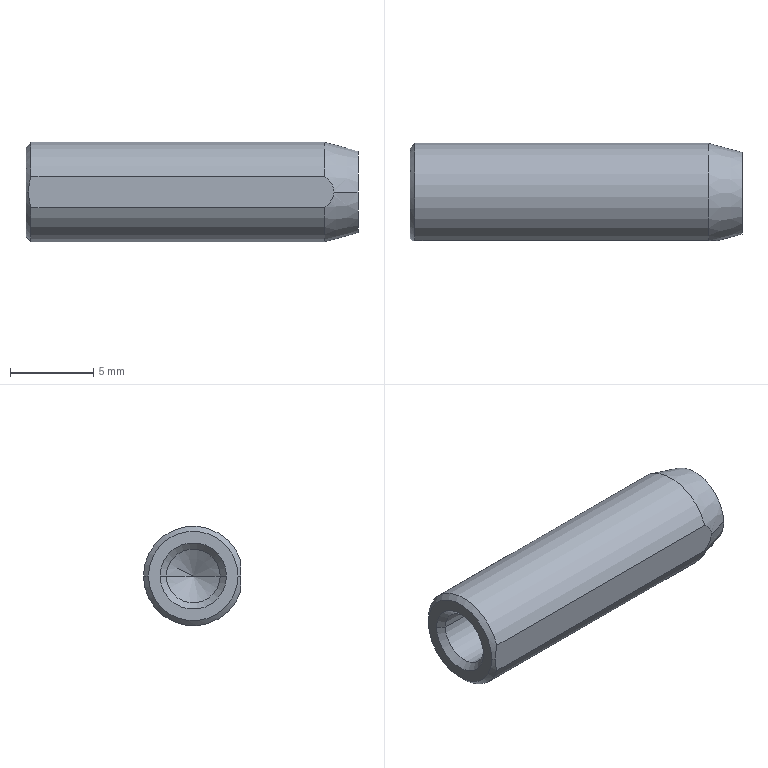Part | STEP file | MSTSS6-20-4 | 1 solid | 15 faces | box 20 x 5.85 x 6 mm | volume 470.29 mm3 | cone 8 | cylinder 4 | plane 3 | commonest cylinder face diameters 3.242 x2 6 x2
STEP:
#1=CARTESIAN_POINT('',(0.,0.,0.));
#2=DIRECTION('',(0.,0.,1.));
#3=DIRECTION('',(1.,0.,0.));
#4=AXIS2_PLACEMENT_3D('',#1,#2,#3);
#5=CARTESIAN_POINT('',(9.464,-1.621,0.));
#6=VERTEX_POINT('',#5);
#7=CARTESIAN_POINT('',(9.464,1.621,0.));
#8=VERTEX_POINT('',#7);
#9=CARTESIAN_POINT('',(9.464,0.,0.));
#10=DIRECTION('',(1.,0.,0.));
#11=DIRECTION('',(0.,1.,0.));
#12=AXIS2_PLACEMENT_3D('',#9,#10,#11);
#13=CIRCLE('',#12,1.621);
#14=CARTESIAN_POINT('',(9.464,0.,0.));
#15=DIRECTION('',(-1.,0.,0.));
#16=DIRECTION('',(0.,-1.,0.));
#17=AXIS2_PLACEMENT_3D('',#14,#15,#16);
#18=CONICAL_SURFACE('',#17,1.621,1.047);
#19=CARTESIAN_POINT('',(9.425,0.));
#20=DIRECTION('',(-1.,0.));
#21=VECTOR('',#20,1.);
#22=LINE('',#19,#21);
#23=(GEOMETRIC_REPRESENTATION_CONTEXT(2)PARAMETRIC_REPRESENTATION_CONTEXT()REPRESENTATION_CONTEXT('',''));
#24=DEFINITIONAL_REPRESENTATION('',(#22),#23);
#25=PCURVE('',#18,#24);
#26=CARTESIAN_POINT('',(10.4,0.,0.));
#27=DIRECTION('',(1.,0.,0.));
#28=DIRECTION('',(0.,1.,0.));
#29=AXIS2_PLACEMENT_3D('',#26,#27,#28);
#30=CYLINDRICAL_SURFACE('',#29,1.621);
#31=CARTESIAN_POINT('',(0.,-0.9359));
#32=DIRECTION('',(1.,0.));
#33=VECTOR('',#32,1.);
#34=LINE('',#31,#33);
#35=(GEOMETRIC_REPRESENTATION_CONTEXT(2)PARAMETRIC_REPRESENTATION_CONTEXT()REPRESENTATION_CONTEXT('',''));
#36=DEFINITIONAL_REPRESENTATION('',(#34),#35);
#37=PCURVE('',#30,#36);
#38=SURFACE_CURVE('',#13,(#25,#37),.PCURVE_S1.);
#39=EDGE_CURVE('',#6,#8,#38,.T.);
#40=ORIENTED_EDGE('',*,*,#39,.T.);
#41=CARTESIAN_POINT('',(10.4,0.,0.));
#42=VERTEX_POINT('',#41);
#43=CARTESIAN_POINT('',(9.464,1.621,0.));
#44=DIRECTION('',(-0.5,0.866,0.));
#45=VECTOR('',#44,1.);
#46=LINE('',#43,#45);
#47=CARTESIAN_POINT('',(3.142,0.));
#48=DIRECTION('',(0.,1.));
#49=VECTOR('',#48,1.);
#50=LINE('',#47,#49);
#51=(GEOMETRIC_REPRESENTATION_CONTEXT(2)PARAMETRIC_REPRESENTATION_CONTEXT()REPRESENTATION_CONTEXT('',''));
#52=DEFINITIONAL_REPRESENTATION('',(#50),#51);
#53=PCURVE('',#18,#52);
#54=CARTESIAN_POINT('',(9.464,0.,0.));
#55=DIRECTION('',(-1.,0.,0.));
#56=DIRECTION('',(0.,-1.,0.));
#57=AXIS2_PLACEMENT_3D('',#54,#55,#56);
#58=CONICAL_SURFACE('',#57,1.621,1.047);
#59=CARTESIAN_POINT('',(3.142,0.));
#60=DIRECTION('',(0.,1.));
#61=VECTOR('',#60,1.);
#62=LINE('',#59,#61);
#63=(GEOMETRIC_REPRESENTATION_CONTEXT(2)PARAMETRIC_REPRESENTATION_CONTEXT()REPRESENTATION_CONTEXT('',''));
#64=DEFINITIONAL_REPRESENTATION('',(#62),#63);
#65=PCURVE('',#58,#64);
#66=SURFACE_CURVE('',#46,(#53,#65),.PCURVE_S1.);
#67=EDGE_CURVE('',#42,#8,#66,.T.);
#68=ORIENTED_EDGE('',*,*,#67,.F.);
#69=CARTESIAN_POINT('',(9.464,-1.621,0.));
#70=DIRECTION('',(-0.5,-0.866,0.));
#71=VECTOR('',#70,1.);
#72=LINE('',#69,#71);
#73=CARTESIAN_POINT('',(6.283,0.));
#74=DIRECTION('',(0.,1.));
#75=VECTOR('',#74,1.);
#76=LINE('',#73,#75);
#77=(GEOMETRIC_REPRESENTATION_CONTEXT(2)PARAMETRIC_REPRESENTATION_CONTEXT()REPRESENTATION_CONTEXT('',''));
#78=DEFINITIONAL_REPRESENTATION('',(#76),#77);
#79=PCURVE('',#18,#78);
#80=CARTESIAN_POINT('',(0.,0.));
#81=DIRECTION('',(0.,1.));
#82=VECTOR('',#81,1.);
#83=LINE('',#80,#82);
#84=(GEOMETRIC_REPRESENTATION_CONTEXT(2)PARAMETRIC_REPRESENTATION_CONTEXT()REPRESENTATION_CONTEXT('',''));
#85=DEFINITIONAL_REPRESENTATION('',(#83),#84);
#86=PCURVE('',#58,#85);
#87=SURFACE_CURVE('',#72,(#79,#86),.PCURVE_S1.);
#88=EDGE_CURVE('',#42,#6,#87,.T.);
#89=ORIENTED_EDGE('',*,*,#88,.T.);
#90=EDGE_LOOP('',(#40,#68,#89));
#91=FACE_BOUND('',#90,.F.);
#92=ADVANCED_FACE('',(#91),#18,.F.);
#93=CARTESIAN_POINT('',(0.379,1.621,0.));
#94=VERTEX_POINT('',#93);
#95=CARTESIAN_POINT('',(10.4,1.621,0.));
#96=DIRECTION('',(1.,0.,0.));
#97=VECTOR('',#96,1.);
#98=LINE('',#95,#97);
#99=CARTESIAN_POINT('',(6.283,0.));
#100=DIRECTION('',(0.,1.));
#101=VECTOR('',#100,1.);
#102=LINE('',#99,#101);
#103=(GEOMETRIC_REPRESENTATION_CONTEXT(2)PARAMETRIC_REPRESENTATION_CONTEXT()REPRESENTATION_CONTEXT('',''));
#104=DEFINITIONAL_REPRESENTATION('',(#102),#103);
#105=PCURVE('',#30,#104);
#106=CARTESIAN_POINT('',(10.4,0.,0.));
#107=DIRECTION('',(1.,0.,0.));
#108=DIRECTION('',(0.,1.,0.));
#109=AXIS2_PLACEMENT_3D('',#106,#107,#108);
#110=CYLINDRICAL_SURFACE('',#109,1.621);
#111=CARTESIAN_POINT('',(0.,0.));
#112=DIRECTION('',(0.,1.));
#113=VECTOR('',#112,1.);
#114=LINE('',#111,#113);
#115=(GEOMETRIC_REPRESENTATION_CONTEXT(2)PARAMETRIC_REPRESENTATION_CONTEXT()REPRESENTATION_CONTEXT('',''));
#116=DEFINITIONAL_REPRESENTATION('',(#114),#115);
#117=PCURVE('',#110,#116);
#118=SURFACE_CURVE('',#98,(#105,#117),.PCURVE_S1.);
#119=EDGE_CURVE('',#94,#8,#118,.T.);
#120=ORIENTED_EDGE('',*,*,#119,.T.);
#121=ORIENTED_EDGE('',*,*,#39,.F.);
#122=CARTESIAN_POINT('',(0.379,-1.621,0.));
#123=VERTEX_POINT('',#122);
#124=CARTESIAN_POINT('',(10.4,-1.621,0.));
#125=DIRECTION('',(1.,0.,0.));
#126=VECTOR('',#125,1.);
#127=LINE('',#124,#126);
#128=CARTESIAN_POINT('',(3.142,0.));
#129=DIRECTION('',(0.,1.));
#130=VECTOR('',#129,1.);
#131=LINE('',#128,#130);
#132=(GEOMETRIC_REPRESENTATION_CONTEXT(2)PARAMETRIC_REPRESENTATION_CONTEXT()REPRESENTATION_CONTEXT('',''));
#133=DEFINITIONAL_REPRESENTATION('',(#131),#132);
#134=PCURVE('',#30,#133);
#135=CARTESIAN_POINT('',(3.142,0.));
#136=DIRECTION('',(0.,1.));
#137=VECTOR('',#136,1.);
#138=LINE('',#135,#137);
#139=(GEOMETRIC_REPRESENTATION_CONTEXT(2)PARAMETRIC_REPRESENTATION_CONTEXT()REPRESENTATION_CONTEXT('',''));
#140=DEFINITIONAL_REPRESENTATION('',(#138),#139);
#141=PCURVE('',#110,#140);
#142=SURFACE_CURVE('',#127,(#134,#141),.PCURVE_S1.);
#143=EDGE_CURVE('',#123,#6,#142,.T.);
#144=ORIENTED_EDGE('',*,*,#143,.F.);
#145=CARTESIAN_POINT('',(0.379,0.,0.));
#146=DIRECTION('',(1.,0.,0.));
#147=DIRECTION('',(0.,1.,0.));
#148=AXIS2_PLACEMENT_3D('',#145,#146,#147);
#149=CIRCLE('',#148,1.621);
#150=CARTESIAN_POINT('',(0.,-10.021));
#151=DIRECTION('',(1.,0.));
#152=VECTOR('',#151,1.);
#153=LINE('',#150,#152);
#154=(GEOMETRIC_REPRESENTATION_CONTEXT(2)PARAMETRIC_REPRESENTATION_CONTEXT()REPRESENTATION_CONTEXT('',''));
#155=DEFINITIONAL_REPRESENTATION('',(#153),#154);
#156=PCURVE('',#30,#155);
#157=CARTESIAN_POINT('',(0.,0.,0.));
#158=DIRECTION('',(-1.,0.,0.));
#159=DIRECTION('',(0.,-1.,0.));
#160=AXIS2_PLACEMENT_3D('',#157,#158,#159);
#161=CONICAL_SURFACE('',#160,2.,0.7854);
#162=CARTESIAN_POINT('',(9.425,-0.379));
#163=DIRECTION('',(-1.,0.));
#164=VECTOR('',#163,1.);
#165=LINE('',#162,#164);
#166=(GEOMETRIC_REPRESENTATION_CONTEXT(2)PARAMETRIC_REPRESENTATION_CONTEXT()REPRESENTATION_CONTEXT('',''));
#167=DEFINITIONAL_REPRESENTATION('',(#165),#166);
#168=PCURVE('',#161,#167);
#169=SURFACE_CURVE('',#149,(#156,#168),.PCURVE_S1.);
#170=EDGE_CURVE('',#123,#94,#169,.T.);
#171=ORIENTED_EDGE('',*,*,#170,.T.);
#172=EDGE_LOOP('',(#120,#121,#144,#171));
#173=FACE_BOUND('',#172,.F.);
#174=ADVANCED_FACE('',(#173),#30,.F.);
#175=CARTESIAN_POINT('',(0.,-2.,0.));
#176=VERTEX_POINT('',#175);
#177=CARTESIAN_POINT('',(0.,-2.,0.));
#178=DIRECTION('',(-0.7071,-0.7071,0.));
#179=VECTOR('',#178,1.);
#180=LINE('',#177,#179);
#181=CARTESIAN_POINT('',(6.283,0.));
#182=DIRECTION('',(0.,1.));
#183=VECTOR('',#182,1.);
#184=LINE('',#181,#183);
#185=(GEOMETRIC_REPRESENTATION_CONTEXT(2)PARAMETRIC_REPRESENTATION_CONTEXT()REPRESENTATION_CONTEXT('',''));
#186=DEFINITIONAL_REPRESENTATION('',(#184),#185);
#187=PCURVE('',#161,#186);
#188=CARTESIAN_POINT('',(0.,0.,0.));
#189=DIRECTION('',(-1.,0.,0.));
#190=DIRECTION('',(0.,-1.,0.));
#191=AXIS2_PLACEMENT_3D('',#188,#189,#190);
#192=CONICAL_SURFACE('',#191,2.,0.7854);
#193=CARTESIAN_POINT('',(0.,0.));
#194=DIRECTION('',(0.,1.));
#195=VECTOR('',#194,1.);
#196=LINE('',#193,#195);
#197=(GEOMETRIC_REPRESENTATION_CONTEXT(2)PARAMETRIC_REPRESENTATION_CONTEXT()REPRESENTATION_CONTEXT('',''));
#198=DEFINITIONAL_REPRESENTATION('',(#196),#197);
#199=PCURVE('',#192,#198);
#200=SURFACE_CURVE('',#180,(#187,#199),.PCURVE_S1.);
#201=EDGE_CURVE('',#123,#176,#200,.T.);
#202=ORIENTED_EDGE('',*,*,#201,.T.);
#203=CARTESIAN_POINT('',(0.,2.,0.));
#204=VERTEX_POINT('',#203);
#205=CARTESIAN_POINT('',(0.,0.,0.));
#206=DIRECTION('',(1.,0.,0.));
#207=DIRECTION('',(0.,1.,0.));
#208=AXIS2_PLACEMENT_3D('',#205,#206,#207);
#209=CIRCLE('',#208,2.);
#210=CARTESIAN_POINT('',(9.425,0.));
#211=DIRECTION('',(-1.,0.));
#212=VECTOR('',#211,1.);
#213=LINE('',#210,#212);
#214=(GEOMETRIC_REPRESENTATION_CONTEXT(2)PARAMETRIC_REPRESENTATION_CONTEXT()REPRESENTATION_CONTEXT('',''));
#215=DEFINITIONAL_REPRESENTATION('',(#213),#214);
#216=PCURVE('',#161,#215);
#217=CARTESIAN_POINT('',(0.,0.,0.));
#218=DIRECTION('',(1.,0.,0.));
#219=DIRECTION('',(0.,1.,0.));
#220=AXIS2_PLACEMENT_3D('',#217,#218,#219);
#221=PLANE('',#220);
#222=CARTESIAN_POINT('',(0.,0.));
#223=DIRECTION('',(1.,0.));
#224=AXIS2_PLACEMENT_2D('',#222,#223);
#225=CIRCLE('',#224,2.);
#226=(GEOMETRIC_REPRESENTATION_CONTEXT(2)PARAMETRIC_REPRESENTATION_CONTEXT()REPRESENTATION_CONTEXT('',''));
#227=DEFINITIONAL_REPRESENTATION('',(#225),#226);
#228=PCURVE('',#221,#227);
#229=SURFACE_CURVE('',#209,(#216,#228),.PCURVE_S1.);
#230=EDGE_CURVE('',#176,#204,#229,.T.);
#231=ORIENTED_EDGE('',*,*,#230,.T.);
#232=CARTESIAN_POINT('',(0.,2.,0.));
#233=DIRECTION('',(-0.7071,0.7071,0.));
#234=VECTOR('',#233,1.);
#235=LINE('',#232,#234);
#236=CARTESIAN_POINT('',(3.142,0.));
#237=DIRECTION('',(0.,1.));
#238=VECTOR('',#237,1.);
#239=LINE('',#236,#238);
#240=(GEOMETRIC_REPRESENTATION_CONTEXT(2)PARAMETRIC_REPRESENTATION_CONTEXT()REPRESENTATION_CONTEXT('',''));
#241=DEFINITIONAL_REPRESENTATION('',(#239),#240);
#242=PCURVE('',#161,#241);
#243=CARTESIAN_POINT('',(3.142,0.));
#244=DIRECTION('',(0.,1.));
#245=VECTOR('',#244,1.);
#246=LINE('',#243,#245);
#247=(GEOMETRIC_REPRESENTATION_CONTEXT(2)PARAMETRIC_REPRESENTATION_CONTEXT()REPRESENTATION_CONTEXT('',''));
#248=DEFINITIONAL_REPRESENTATION('',(#246),#247);
#249=PCURVE('',#192,#248);
#250=SURFACE_CURVE('',#235,(#242,#249),.PCURVE_S1.);
#251=EDGE_CURVE('',#94,#204,#250,.T.);
#252=ORIENTED_EDGE('',*,*,#251,.F.);
#253=ORIENTED_EDGE('',*,*,#170,.F.);
#254=EDGE_LOOP('',(#202,#231,#252,#253));
#255=FACE_BOUND('',#254,.F.);
#256=ADVANCED_FACE('',(#255),#161,.F.);
#257=CARTESIAN_POINT('',(20.,2.464,0.));
#258=VERTEX_POINT('',#257);
#259=CARTESIAN_POINT('',(20.,-2.464,0.));
#260=VERTEX_POINT('',#259);
#261=CARTESIAN_POINT('',(20.,0.,0.));
#262=DIRECTION('',(1.,0.,0.));
#263=DIRECTION('',(0.,1.,0.));
#264=AXIS2_PLACEMENT_3D('',#261,#262,#263);
#265=CIRCLE('',#264,2.464);
#266=CARTESIAN_POINT('',(18.,0.,0.));
#267=DIRECTION('',(-1.,0.,0.));
#268=DIRECTION('',(0.,-1.,0.));
#269=AXIS2_PLACEMENT_3D('',#266,#267,#268);
#270=CONICAL_SURFACE('',#269,3.,0.2618);
#271=CARTESIAN_POINT('',(3.142,-2.));
#272=DIRECTION('',(-1.,0.));
#273=VECTOR('',#272,1.);
#274=LINE('',#271,#273);
#275=(GEOMETRIC_REPRESENTATION_CONTEXT(2)PARAMETRIC_REPRESENTATION_CONTEXT()REPRESENTATION_CONTEXT('',''));
#276=DEFINITIONAL_REPRESENTATION('',(#274),#275);
#277=PCURVE('',#270,#276);
#278=CARTESIAN_POINT('',(20.,0.,2.464));
#279=DIRECTION('',(-1.,0.,0.));
#280=DIRECTION('',(0.,-1.,0.));
#281=AXIS2_PLACEMENT_3D('',#278,#279,#280);
#282=PLANE('',#281);
#283=CARTESIAN_POINT('',(-2.464,-2.464));
#284=CARTESIAN_POINT('',(-2.464,1.804));
#285=CARTESIAN_POINT('',(1.232,-0.3301));
#286=CARTESIAN_POINT('',(4.928,-2.464));
#287=CARTESIAN_POINT('',(1.232,-4.598));
#288=CARTESIAN_POINT('',(-2.464,-6.732));
#289=CARTESIAN_POINT('',(-2.464,-2.464));
#290=(BOUNDED_CURVE()B_SPLINE_CURVE(2,(#283,#284,#285,#286,#287,#288,#289),.UNSPECIFIED.,.T.,.F.)B_SPLINE_CURVE_WITH_KNOTS((1,2,2,2,2,1),(-2.094,0.,2.094,4.189,6.283,8.378),.UNSPECIFIED.)CURVE()GEOMETRIC_REPRESENTATION_ITEM()RATIONAL_B_SPLINE_CURVE((1.,0.5,1.,0.5,1.,0.5,1.))REPRESENTATION_ITEM(''));
#291=(GEOMETRIC_REPRESENTATION_CONTEXT(2)PARAMETRIC_REPRESENTATION_CONTEXT()REPRESENTATION_CONTEXT('',''));
#292=DEFINITIONAL_REPRESENTATION('',(#290),#291);
#293=PCURVE('',#282,#292);
#294=SURFACE_CURVE('',#265,(#277,#293),.PCURVE_S1.);
#295=EDGE_CURVE('',#258,#260,#294,.T.);
#296=ORIENTED_EDGE('',*,*,#295,.F.);
#297=CARTESIAN_POINT('',(18.,3.,0.));
#298=VERTEX_POINT('',#297);
#299=CARTESIAN_POINT('',(18.,3.,0.));
#300=DIRECTION('',(-0.9659,0.2588,0.));
#301=VECTOR('',#300,1.);
#302=LINE('',#299,#301);
#303=CARTESIAN_POINT('',(3.142,0.));
#304=DIRECTION('',(0.,1.));
#305=VECTOR('',#304,1.);
#306=LINE('',#303,#305);
#307=(GEOMETRIC_REPRESENTATION_CONTEXT(2)PARAMETRIC_REPRESENTATION_CONTEXT()REPRESENTATION_CONTEXT('',''));
#308=DEFINITIONAL_REPRESENTATION('',(#306),#307);
#309=PCURVE('',#270,#308);
#310=CARTESIAN_POINT('',(18.,0.,0.));
#311=DIRECTION('',(-1.,0.,0.));
#312=DIRECTION('',(0.,-1.,0.));
#313=AXIS2_PLACEMENT_3D('',#310,#311,#312);
#314=CONICAL_SURFACE('',#313,3.,0.2618);
#315=CARTESIAN_POINT('',(3.142,0.));
#316=DIRECTION('',(0.,1.));
#317=VECTOR('',#316,1.);
#318=LINE('',#315,#317);
#319=(GEOMETRIC_REPRESENTATION_CONTEXT(2)PARAMETRIC_REPRESENTATION_CONTEXT()REPRESENTATION_CONTEXT('',''));
#320=DEFINITIONAL_REPRESENTATION('',(#318),#319);
#321=PCURVE('',#314,#320);
#322=SURFACE_CURVE('',#302,(#309,#321),.PCURVE_S1.);
#323=EDGE_CURVE('',#258,#298,#322,.T.);
#324=ORIENTED_EDGE('',*,*,#323,.T.);
#325=CARTESIAN_POINT('',(18.,-2.85,0.9367));
#326=VERTEX_POINT('',#325);
#327=CARTESIAN_POINT('',(18.,0.,0.));
#328=DIRECTION('',(1.,0.,0.));
#329=DIRECTION('',(0.,1.,0.));
#330=AXIS2_PLACEMENT_3D('',#327,#328,#329);
#331=CIRCLE('',#330,3.);
#332=CARTESIAN_POINT('',(3.142,0.));
#333=DIRECTION('',(-1.,0.));
#334=VECTOR('',#333,1.);
#335=LINE('',#332,#334);
#336=(GEOMETRIC_REPRESENTATION_CONTEXT(2)PARAMETRIC_REPRESENTATION_CONTEXT()REPRESENTATION_CONTEXT('',''));
#337=DEFINITIONAL_REPRESENTATION('',(#335),#336);
#338=PCURVE('',#270,#337);
#339=CARTESIAN_POINT('',(20.,0.,0.));
#340=DIRECTION('',(1.,0.,0.));
#341=DIRECTION('',(0.,1.,0.));
#342=AXIS2_PLACEMENT_3D('',#339,#340,#341);
#343=CYLINDRICAL_SURFACE('',#342,3.);
#344=CARTESIAN_POINT('',(0.,-2.));
#345=DIRECTION('',(1.,0.));
#346=VECTOR('',#345,1.);
#347=LINE('',#344,#346);
#348=(GEOMETRIC_REPRESENTATION_CONTEXT(2)PARAMETRIC_REPRESENTATION_CONTEXT()REPRESENTATION_CONTEXT('',''));
#349=DEFINITIONAL_REPRESENTATION('',(#347),#348);
#350=PCURVE('',#343,#349);
#351=SURFACE_CURVE('',#331,(#338,#350),.PCURVE_S1.);
#352=EDGE_CURVE('',#298,#326,#351,.T.);
#353=ORIENTED_EDGE('',*,*,#352,.T.);
#354=CARTESIAN_POINT('',(18.56,-2.85,0.));
#355=VERTEX_POINT('',#354);
#356=CARTESIAN_POINT('',(18.56,-2.85,0.));
#357=CARTESIAN_POINT('',(18.56,-2.85,0.0942));
#358=CARTESIAN_POINT('',(18.542,-2.85,0.1877));
#359=CARTESIAN_POINT('',(18.478,-2.85,0.365));
#360=CARTESIAN_POINT('',(18.433,-2.85,0.4473));
#361=CARTESIAN_POINT('',(18.275,-2.85,0.682));
#362=CARTESIAN_POINT('',(18.142,-2.85,0.8146));
#363=CARTESIAN_POINT('',(18.,-2.85,0.9367));
#364=B_SPLINE_CURVE_WITH_KNOTS('',3,(#356,#357,#358,#359,#360,#361,#362,#363),.UNSPECIFIED.,.F.,.F.,(4,2,2,4),(0.008062,0.008341,0.00862,0.009177),.UNSPECIFIED.);
#365=CARTESIAN_POINT('',(0.,-0.5598));
#366=CARTESIAN_POINT('',(0.00601,-0.5598));
#367=CARTESIAN_POINT('',(0.01801,-0.5586));
#368=CARTESIAN_POINT('',(0.03591,-0.5534));
#369=CARTESIAN_POINT('',(0.05362,-0.545));
#370=CARTESIAN_POINT('',(0.0711,-0.5333));
#371=CARTESIAN_POINT('',(0.08827,-0.5188));
#372=CARTESIAN_POINT('',(0.1051,-0.5013));
#373=CARTESIAN_POINT('',(0.1214,-0.4814));
#374=CARTESIAN_POINT('',(0.1373,-0.4593));
#375=CARTESIAN_POINT('',(0.1527,-0.435));
#376=CARTESIAN_POINT('',(0.1678,-0.4088));
#377=CARTESIAN_POINT('',(0.1824,-0.3807));
#378=CARTESIAN_POINT('',(0.1967,-0.3511));
#379=CARTESIAN_POINT('',(0.2105,-0.3204));
#380=CARTESIAN_POINT('',(0.2238,-0.2884));
#381=CARTESIAN_POINT('',(0.2368,-0.2554));
#382=CARTESIAN_POINT('',(0.2493,-0.2214));
#383=CARTESIAN_POINT('',(0.2615,-0.1864));
#384=CARTESIAN_POINT('',(0.2733,-0.1506));
#385=CARTESIAN_POINT('',(0.2848,-0.114));
#386=CARTESIAN_POINT('',(0.296,-0.07662));
#387=CARTESIAN_POINT('',(0.3069,-0.03864));
#388=CARTESIAN_POINT('',(0.314,-0.01294));
#389=CARTESIAN_POINT('',(0.3176,0.));
#390=B_SPLINE_CURVE_WITH_KNOTS('',3,(#365,#366,#367,#368,#369,#370,#371,#372,#373,#374,#375,#376,#377,#378,#379,#380,#381,#382,#383,#384,#385,#386,#387,#388,#389),.UNSPECIFIED.,.F.,.F.,(4,1,1,1,1,1,1,1,1,1,1,1,1,1,1,1,1,1,1,1,1,1,4),(0.008062,0.008113,0.008163,0.008214,0.008265,0.008316,0.008366,0.008417,0.008468,0.008518,0.008569,0.00862,0.00867,0.008721,0.008772,0.008822,0.008873,0.008924,0.008974,0.009025,0.009076,0.009126,0.009177),.QUASI_UNIFORM_KNOTS.);
#391=(GEOMETRIC_REPRESENTATION_CONTEXT(2)PARAMETRIC_REPRESENTATION_CONTEXT()REPRESENTATION_CONTEXT('',''));
#392=DEFINITIONAL_REPRESENTATION('',(#390),#391);
#393=PCURVE('',#270,#392);
#394=CARTESIAN_POINT('',(20.,-2.85,-3.));
#395=DIRECTION('',(0.,-1.,0.));
#396=DIRECTION('',(1.,0.,0.));
#397=AXIS2_PLACEMENT_3D('',#394,#395,#396);
#398=PLANE('',#397);
#399=CARTESIAN_POINT('',(-1.44,3.));
#400=CARTESIAN_POINT('',(-1.44,3.094));
#401=CARTESIAN_POINT('',(-1.458,3.188));
#402=CARTESIAN_POINT('',(-1.522,3.365));
#403=CARTESIAN_POINT('',(-1.567,3.447));
#404=CARTESIAN_POINT('',(-1.725,3.682));
#405=CARTESIAN_POINT('',(-1.858,3.815));
#406=CARTESIAN_POINT('',(-2.,3.937));
#407=B_SPLINE_CURVE_WITH_KNOTS('',3,(#399,#400,#401,#402,#403,#404,#405,#406),.UNSPECIFIED.,.F.,.F.,(4,2,2,4),(0.008062,0.008341,0.00862,0.009177),.UNSPECIFIED.);
#408=(GEOMETRIC_REPRESENTATION_CONTEXT(2)PARAMETRIC_REPRESENTATION_CONTEXT()REPRESENTATION_CONTEXT('',''));
#409=DEFINITIONAL_REPRESENTATION('',(#407),#408);
#410=PCURVE('',#398,#409);
#411=SURFACE_CURVE('',#364,(#393,#410),.PCURVE_S1.);
#412=EDGE_CURVE('',#355,#326,#411,.T.);
#413=ORIENTED_EDGE('',*,*,#412,.F.);
#414=CARTESIAN_POINT('',(18.,-3.,0.));
#415=DIRECTION('',(-0.9659,-0.2588,0.));
#416=VECTOR('',#415,1.);
#417=LINE('',#414,#416);
#418=CARTESIAN_POINT('',(0.,0.));
#419=DIRECTION('',(0.,1.));
#420=VECTOR('',#419,1.);
#421=LINE('',#418,#420);
#422=(GEOMETRIC_REPRESENTATION_CONTEXT(2)PARAMETRIC_REPRESENTATION_CONTEXT()REPRESENTATION_CONTEXT('',''));
#423=DEFINITIONAL_REPRESENTATION('',(#421),#422);
#424=PCURVE('',#270,#423);
#425=CARTESIAN_POINT('',(6.283,0.));
#426=DIRECTION('',(0.,1.));
#427=VECTOR('',#426,1.);
#428=LINE('',#425,#427);
#429=(GEOMETRIC_REPRESENTATION_CONTEXT(2)PARAMETRIC_REPRESENTATION_CONTEXT()REPRESENTATION_CONTEXT('',''));
#430=DEFINITIONAL_REPRESENTATION('',(#428),#429);
#431=PCURVE('',#314,#430);
#432=SURFACE_CURVE('',#417,(#424,#431),.PCURVE_S1.);
#433=EDGE_CURVE('',#260,#355,#432,.T.);
#434=ORIENTED_EDGE('',*,*,#433,.F.);
#435=EDGE_LOOP('',(#296,#324,#353,#413,#434));
#436=FACE_BOUND('',#435,.T.);
#437=ADVANCED_FACE('',(#436),#270,.T.);
#438=CARTESIAN_POINT('',(0.3,-2.85,-0.9367));
#439=VERTEX_POINT('',#438);
#440=CARTESIAN_POINT('',(0.3,3.,0.));
#441=VERTEX_POINT('',#440);
#442=CARTESIAN_POINT('',(0.3,0.,0.));
#443=DIRECTION('',(1.,0.,0.));
#444=DIRECTION('',(0.,1.,0.));
#445=AXIS2_PLACEMENT_3D('',#442,#443,#444);
#446=CIRCLE('',#445,3.);
#447=CARTESIAN_POINT('',(20.,0.,0.));
#448=DIRECTION('',(1.,0.,0.));
#449=DIRECTION('',(0.,1.,0.));
#450=AXIS2_PLACEMENT_3D('',#447,#448,#449);
#451=CYLINDRICAL_SURFACE('',#450,3.);
#452=CARTESIAN_POINT('',(0.,-19.7));
#453=DIRECTION('',(1.,0.));
#454=VECTOR('',#453,1.);
#455=LINE('',#452,#454);
#456=(GEOMETRIC_REPRESENTATION_CONTEXT(2)PARAMETRIC_REPRESENTATION_CONTEXT()REPRESENTATION_CONTEXT('',''));
#457=DEFINITIONAL_REPRESENTATION('',(#455),#456);
#458=PCURVE('',#451,#457);
#459=CARTESIAN_POINT('',(0.,0.,0.));
#460=DIRECTION('',(1.,0.,0.));
#461=DIRECTION('',(0.,1.,0.));
#462=AXIS2_PLACEMENT_3D('',#459,#460,#461);
#463=CONICAL_SURFACE('',#462,2.7,0.7854);
#464=CARTESIAN_POINT('',(0.,0.3));
#465=DIRECTION('',(1.,0.));
#466=VECTOR('',#465,1.);
#467=LINE('',#464,#466);
#468=(GEOMETRIC_REPRESENTATION_CONTEXT(2)PARAMETRIC_REPRESENTATION_CONTEXT()REPRESENTATION_CONTEXT('',''));
#469=DEFINITIONAL_REPRESENTATION('',(#467),#468);
#470=PCURVE('',#463,#469);
#471=SURFACE_CURVE('',#446,(#458,#470),.PCURVE_S1.);
#472=EDGE_CURVE('',#439,#441,#471,.T.);
#473=ORIENTED_EDGE('',*,*,#472,.T.);
#474=CARTESIAN_POINT('',(20.,3.,0.));
#475=DIRECTION('',(1.,0.,0.));
#476=VECTOR('',#475,1.);
#477=LINE('',#474,#476);
#478=CARTESIAN_POINT('',(6.283,0.));
#479=DIRECTION('',(0.,1.));
#480=VECTOR('',#479,1.);
#481=LINE('',#478,#480);
#482=(GEOMETRIC_REPRESENTATION_CONTEXT(2)PARAMETRIC_REPRESENTATION_CONTEXT()REPRESENTATION_CONTEXT('',''));
#483=DEFINITIONAL_REPRESENTATION('',(#481),#482);
#484=PCURVE('',#451,#483);
#485=CARTESIAN_POINT('',(0.,0.));
#486=DIRECTION('',(0.,1.));
#487=VECTOR('',#486,1.);
#488=LINE('',#485,#487);
#489=(GEOMETRIC_REPRESENTATION_CONTEXT(2)PARAMETRIC_REPRESENTATION_CONTEXT()REPRESENTATION_CONTEXT('',''));
#490=DEFINITIONAL_REPRESENTATION('',(#488),#489);
#491=PCURVE('',#343,#490);
#492=SURFACE_CURVE('',#477,(#484,#491),.PCURVE_S1.);
#493=EDGE_CURVE('',#441,#298,#492,.T.);
#494=ORIENTED_EDGE('',*,*,#493,.T.);
#495=CARTESIAN_POINT('',(18.,-2.85,-0.9367));
#496=VERTEX_POINT('',#495);
#497=CARTESIAN_POINT('',(18.,0.,0.));
#498=DIRECTION('',(1.,0.,0.));
#499=DIRECTION('',(0.,1.,0.));
#500=AXIS2_PLACEMENT_3D('',#497,#498,#499);
#501=CIRCLE('',#500,3.);
#502=CARTESIAN_POINT('',(0.,-2.));
#503=DIRECTION('',(1.,0.));
#504=VECTOR('',#503,1.);
#505=LINE('',#502,#504);
#506=(GEOMETRIC_REPRESENTATION_CONTEXT(2)PARAMETRIC_REPRESENTATION_CONTEXT()REPRESENTATION_CONTEXT('',''));
#507=DEFINITIONAL_REPRESENTATION('',(#505),#506);
#508=PCURVE('',#451,#507);
#509=CARTESIAN_POINT('',(9.425,0.));
#510=DIRECTION('',(-1.,0.));
#511=VECTOR('',#510,1.);
#512=LINE('',#509,#511);
#513=(GEOMETRIC_REPRESENTATION_CONTEXT(2)PARAMETRIC_REPRESENTATION_CONTEXT()REPRESENTATION_CONTEXT('',''));
#514=DEFINITIONAL_REPRESENTATION('',(#512),#513);
#515=PCURVE('',#314,#514);
#516=SURFACE_CURVE('',#501,(#508,#515),.PCURVE_S1.);
#517=EDGE_CURVE('',#496,#298,#516,.T.);
#518=ORIENTED_EDGE('',*,*,#517,.F.);
#519=CARTESIAN_POINT('',(20.,-2.85,-0.9367));
#520=DIRECTION('',(1.,0.,0.));
#521=VECTOR('',#520,1.);
#522=LINE('',#519,#521);
#523=CARTESIAN_POINT('',(3.459,0.));
#524=DIRECTION('',(0.,1.));
#525=VECTOR('',#524,1.);
#526=LINE('',#523,#525);
#527=(GEOMETRIC_REPRESENTATION_CONTEXT(2)PARAMETRIC_REPRESENTATION_CONTEXT()REPRESENTATION_CONTEXT('',''));
#528=DEFINITIONAL_REPRESENTATION('',(#526),#527);
#529=PCURVE('',#451,#528);
#530=CARTESIAN_POINT('',(0.,2.063));
#531=DIRECTION('',(1.,0.));
#532=VECTOR('',#531,1.);
#533=LINE('',#530,#532);
#534=(GEOMETRIC_REPRESENTATION_CONTEXT(2)PARAMETRIC_REPRESENTATION_CONTEXT()REPRESENTATION_CONTEXT('',''));
#535=DEFINITIONAL_REPRESENTATION('',(#533),#534);
#536=PCURVE('',#398,#535);
#537=SURFACE_CURVE('',#522,(#529,#536),.PCURVE_S1.);
#538=EDGE_CURVE('',#439,#496,#537,.T.);
#539=ORIENTED_EDGE('',*,*,#538,.F.);
#540=EDGE_LOOP('',(#473,#494,#518,#539));
#541=FACE_BOUND('',#540,.T.);
#542=ADVANCED_FACE('',(#541),#451,.T.);
#543=CARTESIAN_POINT('',(0.,2.7,0.));
#544=VERTEX_POINT('',#543);
#545=CARTESIAN_POINT('',(0.,-2.7,0.));
#546=VERTEX_POINT('',#545);
#547=CARTESIAN_POINT('',(0.,0.,0.));
#548=DIRECTION('',(1.,0.,0.));
#549=DIRECTION('',(0.,1.,0.));
#550=AXIS2_PLACEMENT_3D('',#547,#548,#549);
#551=CIRCLE('',#550,2.7);
#552=CARTESIAN_POINT('',(0.,0.,0.));
#553=DIRECTION('',(1.,0.,0.));
#554=DIRECTION('',(0.,1.,0.));
#555=AXIS2_PLACEMENT_3D('',#552,#553,#554);
#556=CONICAL_SURFACE('',#555,2.7,0.7854);
#557=CARTESIAN_POINT('',(0.,0.));
#558=DIRECTION('',(1.,0.));
#559=VECTOR('',#558,1.);
#560=LINE('',#557,#559);
#561=(GEOMETRIC_REPRESENTATION_CONTEXT(2)PARAMETRIC_REPRESENTATION_CONTEXT()REPRESENTATION_CONTEXT('',''));
#562=DEFINITIONAL_REPRESENTATION('',(#560),#561);
#563=PCURVE('',#556,#562);
#564=CARTESIAN_POINT('',(0.,0.));
#565=DIRECTION('',(1.,0.));
#566=AXIS2_PLACEMENT_2D('',#564,#565);
#567=CIRCLE('',#566,2.7);
#568=(GEOMETRIC_REPRESENTATION_CONTEXT(2)PARAMETRIC_REPRESENTATION_CONTEXT()REPRESENTATION_CONTEXT('',''));
#569=DEFINITIONAL_REPRESENTATION('',(#567),#568);
#570=PCURVE('',#221,#569);
#571=SURFACE_CURVE('',#551,(#563,#570),.PCURVE_S1.);
#572=EDGE_CURVE('',#544,#546,#571,.T.);
#573=ORIENTED_EDGE('',*,*,#572,.T.);
#574=CARTESIAN_POINT('',(0.15,-2.85,0.));
#575=VERTEX_POINT('',#574);
#576=CARTESIAN_POINT('',(0.,-2.7,0.));
#577=DIRECTION('',(0.7071,-0.7071,0.));
#578=VECTOR('',#577,1.);
#579=LINE('',#576,#578);
#580=CARTESIAN_POINT('',(3.142,0.));
#581=DIRECTION('',(0.,1.));
#582=VECTOR('',#581,1.);
#583=LINE('',#580,#582);
#584=(GEOMETRIC_REPRESENTATION_CONTEXT(2)PARAMETRIC_REPRESENTATION_CONTEXT()REPRESENTATION_CONTEXT('',''));
#585=DEFINITIONAL_REPRESENTATION('',(#583),#584);
#586=PCURVE('',#556,#585);
#587=CARTESIAN_POINT('',(3.142,0.));
#588=DIRECTION('',(0.,1.));
#589=VECTOR('',#588,1.);
#590=LINE('',#587,#589);
#591=(GEOMETRIC_REPRESENTATION_CONTEXT(2)PARAMETRIC_REPRESENTATION_CONTEXT()REPRESENTATION_CONTEXT('',''));
#592=DEFINITIONAL_REPRESENTATION('',(#590),#591);
#593=PCURVE('',#463,#592);
#594=SURFACE_CURVE('',#579,(#586,#593),.PCURVE_S1.);
#595=EDGE_CURVE('',#546,#575,#594,.T.);
#596=ORIENTED_EDGE('',*,*,#595,.T.);
#597=CARTESIAN_POINT('',(0.3,-2.85,0.9367));
#598=VERTEX_POINT('',#597);
#599=CARTESIAN_POINT('',(0.3,-2.85,0.9367));
#600=CARTESIAN_POINT('',(0.205,-2.85,0.6325));
#601=CARTESIAN_POINT('',(0.15,-2.85,0.3209));
#602=CARTESIAN_POINT('',(0.15,-2.85,0.));
#603=B_SPLINE_CURVE_WITH_KNOTS('',3,(#599,#600,#601,#602),.UNSPECIFIED.,.F.,.F.,(4,4),(0.009751,0.01068),.PIECEWISE_BEZIER_KNOTS.);
#604=CARTESIAN_POINT('',(2.824,0.3));
#605=CARTESIAN_POINT('',(2.828,0.2957));
#606=CARTESIAN_POINT('',(2.837,0.2872));
#607=CARTESIAN_POINT('',(2.851,0.275));
#608=CARTESIAN_POINT('',(2.864,0.2633));
#609=CARTESIAN_POINT('',(2.878,0.2521));
#610=CARTESIAN_POINT('',(2.891,0.2415));
#611=CARTESIAN_POINT('',(2.905,0.2314));
#612=CARTESIAN_POINT('',(2.919,0.2218));
#613=CARTESIAN_POINT('',(2.933,0.2128));
#614=CARTESIAN_POINT('',(2.948,0.2044));
#615=CARTESIAN_POINT('',(2.962,0.1965));
#616=CARTESIAN_POINT('',(2.977,0.1892));
#617=CARTESIAN_POINT('',(2.991,0.1825));
#618=CARTESIAN_POINT('',(3.006,0.1764));
#619=CARTESIAN_POINT('',(3.021,0.1709));
#620=CARTESIAN_POINT('',(3.035,0.1661));
#621=CARTESIAN_POINT('',(3.05,0.1618));
#622=CARTESIAN_POINT('',(3.065,0.1582));
#623=CARTESIAN_POINT('',(3.081,0.1552));
#624=CARTESIAN_POINT('',(3.096,0.1529));
#625=CARTESIAN_POINT('',(3.111,0.1512));
#626=CARTESIAN_POINT('',(3.126,0.1502));
#627=CARTESIAN_POINT('',(3.136,0.15));
#628=CARTESIAN_POINT('',(3.142,0.15));
#629=B_SPLINE_CURVE_WITH_KNOTS('',3,(#604,#605,#606,#607,#608,#609,#610,#611,#612,#613,#614,#615,#616,#617,#618,#619,#620,#621,#622,#623,#624,#625,#626,#627,#628),.UNSPECIFIED.,.F.,.F.,(4,1,1,1,1,1,1,1,1,1,1,1,1,1,1,1,1,1,1,1,1,1,4),(0.009751,0.009793,0.009835,0.009877,0.00992,0.009962,0.01,0.01005,0.01009,0.01013,0.01017,0.01022,0.01026,0.0103,0.01034,0.01038,0.01043,0.01047,0.01051,0.01055,0.0106,0.01064,0.01068),.QUASI_UNIFORM_KNOTS.);
#630=(GEOMETRIC_REPRESENTATION_CONTEXT(2)PARAMETRIC_REPRESENTATION_CONTEXT()REPRESENTATION_CONTEXT('',''));
#631=DEFINITIONAL_REPRESENTATION('',(#629),#630);
#632=PCURVE('',#556,#631);
#633=CARTESIAN_POINT('',(-19.7,3.937));
#634=CARTESIAN_POINT('',(-19.795,3.632));
#635=CARTESIAN_POINT('',(-19.85,3.321));
#636=CARTESIAN_POINT('',(-19.85,3.));
#637=B_SPLINE_CURVE_WITH_KNOTS('',3,(#633,#634,#635,#636),.UNSPECIFIED.,.F.,.F.,(4,4),(0.009751,0.01068),.PIECEWISE_BEZIER_KNOTS.);
#638=(GEOMETRIC_REPRESENTATION_CONTEXT(2)PARAMETRIC_REPRESENTATION_CONTEXT()REPRESENTATION_CONTEXT('',''));
#639=DEFINITIONAL_REPRESENTATION('',(#637),#638);
#640=PCURVE('',#398,#639);
#641=SURFACE_CURVE('',#603,(#632,#640),.PCURVE_S1.);
#642=EDGE_CURVE('',#598,#575,#641,.T.);
#643=ORIENTED_EDGE('',*,*,#642,.F.);
#644=CARTESIAN_POINT('',(0.3,0.,0.));
#645=DIRECTION('',(1.,0.,0.));
#646=DIRECTION('',(0.,1.,0.));
#647=AXIS2_PLACEMENT_3D('',#644,#645,#646);
#648=CIRCLE('',#647,3.);
#649=CARTESIAN_POINT('',(0.,0.3));
#650=DIRECTION('',(1.,0.));
#651=VECTOR('',#650,1.);
#652=LINE('',#649,#651);
#653=(GEOMETRIC_REPRESENTATION_CONTEXT(2)PARAMETRIC_REPRESENTATION_CONTEXT()REPRESENTATION_CONTEXT('',''));
#654=DEFINITIONAL_REPRESENTATION('',(#652),#653);
#655=PCURVE('',#556,#654);
#656=CARTESIAN_POINT('',(0.,-19.7));
#657=DIRECTION('',(1.,0.));
#658=VECTOR('',#657,1.);
#659=LINE('',#656,#658);
#660=(GEOMETRIC_REPRESENTATION_CONTEXT(2)PARAMETRIC_REPRESENTATION_CONTEXT()REPRESENTATION_CONTEXT('',''));
#661=DEFINITIONAL_REPRESENTATION('',(#659),#660);
#662=PCURVE('',#343,#661);
#663=SURFACE_CURVE('',#648,(#655,#662),.PCURVE_S1.);
#664=EDGE_CURVE('',#441,#598,#663,.T.);
#665=ORIENTED_EDGE('',*,*,#664,.F.);
#666=CARTESIAN_POINT('',(0.,2.7,0.));
#667=DIRECTION('',(0.7071,0.7071,0.));
#668=VECTOR('',#667,1.);
#669=LINE('',#666,#668);
#670=CARTESIAN_POINT('',(0.,0.));
#671=DIRECTION('',(0.,1.));
#672=VECTOR('',#671,1.);
#673=LINE('',#670,#672);
#674=(GEOMETRIC_REPRESENTATION_CONTEXT(2)PARAMETRIC_REPRESENTATION_CONTEXT()REPRESENTATION_CONTEXT('',''));
#675=DEFINITIONAL_REPRESENTATION('',(#673),#674);
#676=PCURVE('',#556,#675);
#677=CARTESIAN_POINT('',(6.283,0.));
#678=DIRECTION('',(0.,1.));
#679=VECTOR('',#678,1.);
#680=LINE('',#677,#679);
#681=(GEOMETRIC_REPRESENTATION_CONTEXT(2)PARAMETRIC_REPRESENTATION_CONTEXT()REPRESENTATION_CONTEXT('',''));
#682=DEFINITIONAL_REPRESENTATION('',(#680),#681);
#683=PCURVE('',#463,#682);
#684=SURFACE_CURVE('',#669,(#676,#683),.PCURVE_S1.);
#685=EDGE_CURVE('',#544,#441,#684,.T.);
#686=ORIENTED_EDGE('',*,*,#685,.F.);
#687=EDGE_LOOP('',(#573,#596,#643,#665,#686));
#688=FACE_BOUND('',#687,.T.);
#689=ADVANCED_FACE('',(#688),#556,.T.);
#690=ORIENTED_EDGE('',*,*,#595,.F.);
#691=CARTESIAN_POINT('',(0.,0.,0.));
#692=DIRECTION('',(1.,0.,0.));
#693=DIRECTION('',(0.,1.,0.));
#694=AXIS2_PLACEMENT_3D('',#691,#692,#693);
#695=CIRCLE('',#694,2.7);
#696=CARTESIAN_POINT('',(0.,0.));
#697=DIRECTION('',(1.,0.));
#698=VECTOR('',#697,1.);
#699=LINE('',#696,#698);
#700=(GEOMETRIC_REPRESENTATION_CONTEXT(2)PARAMETRIC_REPRESENTATION_CONTEXT()REPRESENTATION_CONTEXT('',''));
#701=DEFINITIONAL_REPRESENTATION('',(#699),#700);
#702=PCURVE('',#463,#701);
#703=CARTESIAN_POINT('',(0.,0.));
#704=DIRECTION('',(1.,0.));
#705=AXIS2_PLACEMENT_2D('',#703,#704);
#706=CIRCLE('',#705,2.7);
#707=(GEOMETRIC_REPRESENTATION_CONTEXT(2)PARAMETRIC_REPRESENTATION_CONTEXT()REPRESENTATION_CONTEXT('',''));
#708=DEFINITIONAL_REPRESENTATION('',(#706),#707);
#709=PCURVE('',#221,#708);
#710=SURFACE_CURVE('',#695,(#702,#709),.PCURVE_S1.);
#711=EDGE_CURVE('',#546,#544,#710,.T.);
#712=ORIENTED_EDGE('',*,*,#711,.T.);
#713=ORIENTED_EDGE('',*,*,#685,.T.);
#714=ORIENTED_EDGE('',*,*,#472,.F.);
#715=CARTESIAN_POINT('',(0.15,-2.85,0.));
#716=CARTESIAN_POINT('',(0.15,-2.85,-0.321));
#717=CARTESIAN_POINT('',(0.205,-2.85,-0.6324));
#718=CARTESIAN_POINT('',(0.3,-2.85,-0.9367));
#719=B_SPLINE_CURVE_WITH_KNOTS('',3,(#715,#716,#717,#718),.UNSPECIFIED.,.F.,.F.,(4,4),(0.01068,0.01161),.PIECEWISE_BEZIER_KNOTS.);
#720=CARTESIAN_POINT('',(3.142,0.15));
#721=CARTESIAN_POINT('',(3.147,0.15));
#722=CARTESIAN_POINT('',(3.157,0.1502));
#723=CARTESIAN_POINT('',(3.172,0.1512));
#724=CARTESIAN_POINT('',(3.187,0.1529));
#725=CARTESIAN_POINT('',(3.203,0.1552));
#726=CARTESIAN_POINT('',(3.218,0.1582));
#727=CARTESIAN_POINT('',(3.233,0.1618));
#728=CARTESIAN_POINT('',(3.248,0.1661));
#729=CARTESIAN_POINT('',(3.263,0.1709));
#730=CARTESIAN_POINT('',(3.277,0.1764));
#731=CARTESIAN_POINT('',(3.292,0.1825));
#732=CARTESIAN_POINT('',(3.307,0.1892));
#733=CARTESIAN_POINT('',(3.321,0.1965));
#734=CARTESIAN_POINT('',(3.335,0.2044));
#735=CARTESIAN_POINT('',(3.35,0.2128));
#736=CARTESIAN_POINT('',(3.364,0.2218));
#737=CARTESIAN_POINT('',(3.378,0.2314));
#738=CARTESIAN_POINT('',(3.392,0.2415));
#739=CARTESIAN_POINT('',(3.405,0.2521));
#740=CARTESIAN_POINT('',(3.419,0.2633));
#741=CARTESIAN_POINT('',(3.433,0.275));
#742=CARTESIAN_POINT('',(3.446,0.2872));
#743=CARTESIAN_POINT('',(3.455,0.2957));
#744=CARTESIAN_POINT('',(3.459,0.3));
#745=B_SPLINE_CURVE_WITH_KNOTS('',3,(#720,#721,#722,#723,#724,#725,#726,#727,#728,#729,#730,#731,#732,#733,#734,#735,#736,#737,#738,#739,#740,#741,#742,#743,#744),.UNSPECIFIED.,.F.,.F.,(4,1,1,1,1,1,1,1,1,1,1,1,1,1,1,1,1,1,1,1,1,1,4),(0.01068,0.01072,0.01077,0.01081,0.01085,0.01089,0.01093,0.01098,0.01102,0.01106,0.0111,0.01115,0.01119,0.01123,0.01127,0.01132,0.01136,0.0114,0.01144,0.01148,0.01153,0.01157,0.01161),.QUASI_UNIFORM_KNOTS.);
#746=(GEOMETRIC_REPRESENTATION_CONTEXT(2)PARAMETRIC_REPRESENTATION_CONTEXT()REPRESENTATION_CONTEXT('',''));
#747=DEFINITIONAL_REPRESENTATION('',(#745),#746);
#748=PCURVE('',#463,#747);
#749=CARTESIAN_POINT('',(-19.85,3.));
#750=CARTESIAN_POINT('',(-19.85,2.679));
#751=CARTESIAN_POINT('',(-19.795,2.368));
#752=CARTESIAN_POINT('',(-19.7,2.063));
#753=B_SPLINE_CURVE_WITH_KNOTS('',3,(#749,#750,#751,#752),.UNSPECIFIED.,.F.,.F.,(4,4),(0.01068,0.01161),.PIECEWISE_BEZIER_KNOTS.);
#754=(GEOMETRIC_REPRESENTATION_CONTEXT(2)PARAMETRIC_REPRESENTATION_CONTEXT()REPRESENTATION_CONTEXT('',''));
#755=DEFINITIONAL_REPRESENTATION('',(#753),#754);
#756=PCURVE('',#398,#755);
#757=SURFACE_CURVE('',#719,(#748,#756),.PCURVE_S1.);
#758=EDGE_CURVE('',#575,#439,#757,.T.);
#759=ORIENTED_EDGE('',*,*,#758,.F.);
#760=EDGE_LOOP('',(#690,#712,#713,#714,#759));
#761=FACE_BOUND('',#760,.T.);
#762=ADVANCED_FACE('',(#761),#463,.T.);
#763=ORIENTED_EDGE('',*,*,#493,.F.);
#764=ORIENTED_EDGE('',*,*,#664,.T.);
#765=CARTESIAN_POINT('',(20.,-2.85,0.9367));
#766=DIRECTION('',(-1.,0.,0.));
#767=VECTOR('',#766,1.);
#768=LINE('',#765,#767);
#769=CARTESIAN_POINT('',(2.824,0.));
#770=DIRECTION('',(0.,-1.));
#771=VECTOR('',#770,1.);
#772=LINE('',#769,#771);
#773=(GEOMETRIC_REPRESENTATION_CONTEXT(2)PARAMETRIC_REPRESENTATION_CONTEXT()REPRESENTATION_CONTEXT('',''));
#774=DEFINITIONAL_REPRESENTATION('',(#772),#773);
#775=PCURVE('',#343,#774);
#776=CARTESIAN_POINT('',(0.,3.937));
#777=DIRECTION('',(-1.,0.));
#778=VECTOR('',#777,1.);
#779=LINE('',#776,#778);
#780=(GEOMETRIC_REPRESENTATION_CONTEXT(2)PARAMETRIC_REPRESENTATION_CONTEXT()REPRESENTATION_CONTEXT('',''));
#781=DEFINITIONAL_REPRESENTATION('',(#779),#780);
#782=PCURVE('',#398,#781);
#783=SURFACE_CURVE('',#768,(#775,#782),.PCURVE_S1.);
#784=EDGE_CURVE('',#326,#598,#783,.T.);
#785=ORIENTED_EDGE('',*,*,#784,.F.);
#786=ORIENTED_EDGE('',*,*,#352,.F.);
#787=EDGE_LOOP('',(#763,#764,#785,#786));
#788=FACE_BOUND('',#787,.T.);
#789=ADVANCED_FACE('',(#788),#343,.T.);
#790=ORIENTED_EDGE('',*,*,#323,.F.);
#791=CARTESIAN_POINT('',(20.,0.,0.));
#792=DIRECTION('',(1.,0.,0.));
#793=DIRECTION('',(0.,1.,0.));
#794=AXIS2_PLACEMENT_3D('',#791,#792,#793);
#795=CIRCLE('',#794,2.464);
#796=CARTESIAN_POINT('',(9.425,-2.));
#797=DIRECTION('',(-1.,0.));
#798=VECTOR('',#797,1.);
#799=LINE('',#796,#798);
#800=(GEOMETRIC_REPRESENTATION_CONTEXT(2)PARAMETRIC_REPRESENTATION_CONTEXT()REPRESENTATION_CONTEXT('',''));
#801=DEFINITIONAL_REPRESENTATION('',(#799),#800);
#802=PCURVE('',#314,#801);
#803=CARTESIAN_POINT('',(-2.464,-2.464));
#804=CARTESIAN_POINT('',(-2.464,1.804));
#805=CARTESIAN_POINT('',(1.232,-0.3301));
#806=CARTESIAN_POINT('',(4.928,-2.464));
#807=CARTESIAN_POINT('',(1.232,-4.598));
#808=CARTESIAN_POINT('',(-2.464,-6.732));
#809=CARTESIAN_POINT('',(-2.464,-2.464));
#810=(BOUNDED_CURVE()B_SPLINE_CURVE(2,(#803,#804,#805,#806,#807,#808,#809),.UNSPECIFIED.,.T.,.F.)B_SPLINE_CURVE_WITH_KNOTS((1,2,2,2,2,1),(-2.094,0.,2.094,4.189,6.283,8.378),.UNSPECIFIED.)CURVE()GEOMETRIC_REPRESENTATION_ITEM()RATIONAL_B_SPLINE_CURVE((1.,0.5,1.,0.5,1.,0.5,1.))REPRESENTATION_ITEM(''));
#811=(GEOMETRIC_REPRESENTATION_CONTEXT(2)PARAMETRIC_REPRESENTATION_CONTEXT()REPRESENTATION_CONTEXT('',''));
#812=DEFINITIONAL_REPRESENTATION('',(#810),#811);
#813=PCURVE('',#282,#812);
#814=SURFACE_CURVE('',#795,(#802,#813),.PCURVE_S1.);
#815=EDGE_CURVE('',#260,#258,#814,.T.);
#816=ORIENTED_EDGE('',*,*,#815,.F.);
#817=ORIENTED_EDGE('',*,*,#433,.T.);
#818=CARTESIAN_POINT('',(18.,-2.85,-0.9367));
#819=CARTESIAN_POINT('',(18.142,-2.85,-0.8152));
#820=CARTESIAN_POINT('',(18.275,-2.85,-0.6804));
#821=CARTESIAN_POINT('',(18.432,-2.85,-0.4498));
#822=CARTESIAN_POINT('',(18.477,-2.85,-0.3665));
#823=CARTESIAN_POINT('',(18.542,-2.85,-0.1886));
#824=CARTESIAN_POINT('',(18.56,-2.85,-0.09452));
#825=CARTESIAN_POINT('',(18.56,-2.85,0.));
#826=B_SPLINE_CURVE_WITH_KNOTS('',3,(#818,#819,#820,#821,#822,#823,#824,#825),.UNSPECIFIED.,.F.,.F.,(4,2,2,4),(0.006943,0.007503,0.007782,0.008062),.UNSPECIFIED.);
#827=CARTESIAN_POINT('',(5.966,0.));
#828=CARTESIAN_POINT('',(5.969,-0.01288));
#829=CARTESIAN_POINT('',(5.976,-0.0385));
#830=CARTESIAN_POINT('',(5.987,-0.07644));
#831=CARTESIAN_POINT('',(5.998,-0.1138));
#832=CARTESIAN_POINT('',(6.01,-0.1505));
#833=CARTESIAN_POINT('',(6.022,-0.1864));
#834=CARTESIAN_POINT('',(6.034,-0.2214));
#835=CARTESIAN_POINT('',(6.047,-0.2555));
#836=CARTESIAN_POINT('',(6.059,-0.2885));
#837=CARTESIAN_POINT('',(6.073,-0.3203));
#838=CARTESIAN_POINT('',(6.086,-0.3508));
#839=CARTESIAN_POINT('',(6.1,-0.38));
#840=CARTESIAN_POINT('',(6.115,-0.4077));
#841=CARTESIAN_POINT('',(6.13,-0.4339));
#842=CARTESIAN_POINT('',(6.145,-0.4583));
#843=CARTESIAN_POINT('',(6.161,-0.4807));
#844=CARTESIAN_POINT('',(6.178,-0.5008));
#845=CARTESIAN_POINT('',(6.195,-0.5184));
#846=CARTESIAN_POINT('',(6.212,-0.5331));
#847=CARTESIAN_POINT('',(6.229,-0.5448));
#848=CARTESIAN_POINT('',(6.247,-0.5534));
#849=CARTESIAN_POINT('',(6.265,-0.5586));
#850=CARTESIAN_POINT('',(6.277,-0.5598));
#851=CARTESIAN_POINT('',(6.283,-0.5598));
#852=B_SPLINE_CURVE_WITH_KNOTS('',3,(#827,#828,#829,#830,#831,#832,#833,#834,#835,#836,#837,#838,#839,#840,#841,#842,#843,#844,#845,#846,#847,#848,#849,#850,#851),.UNSPECIFIED.,.F.,.F.,(4,1,1,1,1,1,1,1,1,1,1,1,1,1,1,1,1,1,1,1,1,1,4),(0.006943,0.006994,0.007045,0.007096,0.007147,0.007198,0.007248,0.007299,0.00735,0.007401,0.007452,0.007503,0.007554,0.007604,0.007655,0.007706,0.007757,0.007808,0.007859,0.00791,0.00796,0.008011,0.008062),.QUASI_UNIFORM_KNOTS.);
#853=(GEOMETRIC_REPRESENTATION_CONTEXT(2)PARAMETRIC_REPRESENTATION_CONTEXT()REPRESENTATION_CONTEXT('',''));
#854=DEFINITIONAL_REPRESENTATION('',(#852),#853);
#855=PCURVE('',#314,#854);
#856=CARTESIAN_POINT('',(-2.,2.063));
#857=CARTESIAN_POINT('',(-1.858,2.185));
#858=CARTESIAN_POINT('',(-1.725,2.32));
#859=CARTESIAN_POINT('',(-1.568,2.55));
#860=CARTESIAN_POINT('',(-1.523,2.633));
#861=CARTESIAN_POINT('',(-1.458,2.811));
#862=CARTESIAN_POINT('',(-1.44,2.905));
#863=CARTESIAN_POINT('',(-1.44,3.));
#864=B_SPLINE_CURVE_WITH_KNOTS('',3,(#856,#857,#858,#859,#860,#861,#862,#863),.UNSPECIFIED.,.F.,.F.,(4,2,2,4),(0.006943,0.007503,0.007782,0.008062),.UNSPECIFIED.);
#865=(GEOMETRIC_REPRESENTATION_CONTEXT(2)PARAMETRIC_REPRESENTATION_CONTEXT()REPRESENTATION_CONTEXT('',''));
#866=DEFINITIONAL_REPRESENTATION('',(#864),#865);
#867=PCURVE('',#398,#866);
#868=SURFACE_CURVE('',#826,(#855,#867),.PCURVE_S1.);
#869=EDGE_CURVE('',#496,#355,#868,.T.);
#870=ORIENTED_EDGE('',*,*,#869,.F.);
#871=ORIENTED_EDGE('',*,*,#517,.T.);
#872=EDGE_LOOP('',(#790,#816,#817,#870,#871));
#873=FACE_BOUND('',#872,.T.);
#874=ADVANCED_FACE('',(#873),#314,.T.);
#875=ORIENTED_EDGE('',*,*,#572,.F.);
#876=ORIENTED_EDGE('',*,*,#711,.F.);
#877=EDGE_LOOP('',(#875,#876));
#878=FACE_BOUND('',#877,.T.);
#879=ORIENTED_EDGE('',*,*,#230,.T.);
#880=CARTESIAN_POINT('',(0.,0.,0.));
#881=DIRECTION('',(1.,0.,0.));
#882=DIRECTION('',(0.,1.,0.));
#883=AXIS2_PLACEMENT_3D('',#880,#881,#882);
#884=CIRCLE('',#883,2.);
#885=CARTESIAN_POINT('',(0.,0.));
#886=DIRECTION('',(1.,0.));
#887=AXIS2_PLACEMENT_2D('',#885,#886);
#888=CIRCLE('',#887,2.);
#889=(GEOMETRIC_REPRESENTATION_CONTEXT(2)PARAMETRIC_REPRESENTATION_CONTEXT()REPRESENTATION_CONTEXT('',''));
#890=DEFINITIONAL_REPRESENTATION('',(#888),#889);
#891=PCURVE('',#221,#890);
#892=CARTESIAN_POINT('',(3.142,0.));
#893=DIRECTION('',(-1.,0.));
#894=VECTOR('',#893,1.);
#895=LINE('',#892,#894);
#896=(GEOMETRIC_REPRESENTATION_CONTEXT(2)PARAMETRIC_REPRESENTATION_CONTEXT()REPRESENTATION_CONTEXT('',''));
#897=DEFINITIONAL_REPRESENTATION('',(#895),#896);
#898=PCURVE('',#192,#897);
#899=SURFACE_CURVE('',#884,(#891,#898),.PCURVE_S1.);
#900=EDGE_CURVE('',#204,#176,#899,.T.);
#901=ORIENTED_EDGE('',*,*,#900,.T.);
#902=EDGE_LOOP('',(#879,#901));
#903=FACE_BOUND('',#902,.T.);
#904=ADVANCED_FACE('',(#878,#903),#221,.F.);
#905=ORIENTED_EDGE('',*,*,#815,.T.);
#906=ORIENTED_EDGE('',*,*,#295,.T.);
#907=EDGE_LOOP('',(#905,#906));
#908=FACE_BOUND('',#907,.T.);
#909=ADVANCED_FACE('',(#908),#282,.F.);
#910=ORIENTED_EDGE('',*,*,#900,.T.);
#911=ORIENTED_EDGE('',*,*,#201,.F.);
#912=CARTESIAN_POINT('',(0.379,0.,0.));
#913=DIRECTION('',(1.,0.,0.));
#914=DIRECTION('',(0.,1.,0.));
#915=AXIS2_PLACEMENT_3D('',#912,#913,#914);
#916=CIRCLE('',#915,1.621);
#917=CARTESIAN_POINT('',(3.142,-0.379));
#918=DIRECTION('',(-1.,0.));
#919=VECTOR('',#918,1.);
#920=LINE('',#917,#919);
#921=(GEOMETRIC_REPRESENTATION_CONTEXT(2)PARAMETRIC_REPRESENTATION_CONTEXT()REPRESENTATION_CONTEXT('',''));
#922=DEFINITIONAL_REPRESENTATION('',(#920),#921);
#923=PCURVE('',#192,#922);
#924=CARTESIAN_POINT('',(0.,-10.021));
#925=DIRECTION('',(1.,0.));
#926=VECTOR('',#925,1.);
#927=LINE('',#924,#926);
#928=(GEOMETRIC_REPRESENTATION_CONTEXT(2)PARAMETRIC_REPRESENTATION_CONTEXT()REPRESENTATION_CONTEXT('',''));
#929=DEFINITIONAL_REPRESENTATION('',(#927),#928);
#930=PCURVE('',#110,#929);
#931=SURFACE_CURVE('',#916,(#923,#930),.PCURVE_S1.);
#932=EDGE_CURVE('',#94,#123,#931,.T.);
#933=ORIENTED_EDGE('',*,*,#932,.F.);
#934=ORIENTED_EDGE('',*,*,#251,.T.);
#935=EDGE_LOOP('',(#910,#911,#933,#934));
#936=FACE_BOUND('',#935,.F.);
#937=ADVANCED_FACE('',(#936),#192,.F.);
#938=CARTESIAN_POINT('',(9.464,0.,0.));
#939=DIRECTION('',(1.,0.,0.));
#940=DIRECTION('',(0.,1.,0.));
#941=AXIS2_PLACEMENT_3D('',#938,#939,#940);
#942=CIRCLE('',#941,1.621);
#943=CARTESIAN_POINT('',(0.,-0.9359));
#944=DIRECTION('',(1.,0.));
#945=VECTOR('',#944,1.);
#946=LINE('',#943,#945);
#947=(GEOMETRIC_REPRESENTATION_CONTEXT(2)PARAMETRIC_REPRESENTATION_CONTEXT()REPRESENTATION_CONTEXT('',''));
#948=DEFINITIONAL_REPRESENTATION('',(#946),#947);
#949=PCURVE('',#110,#948);
#950=CARTESIAN_POINT('',(3.142,0.));
#951=DIRECTION('',(-1.,0.));
#952=VECTOR('',#951,1.);
#953=LINE('',#950,#952);
#954=(GEOMETRIC_REPRESENTATION_CONTEXT(2)PARAMETRIC_REPRESENTATION_CONTEXT()REPRESENTATION_CONTEXT('',''));
#955=DEFINITIONAL_REPRESENTATION('',(#953),#954);
#956=PCURVE('',#58,#955);
#957=SURFACE_CURVE('',#942,(#949,#956),.PCURVE_S1.);
#958=EDGE_CURVE('',#8,#6,#957,.T.);
#959=ORIENTED_EDGE('',*,*,#958,.F.);
#960=ORIENTED_EDGE('',*,*,#119,.F.);
#961=ORIENTED_EDGE('',*,*,#932,.T.);
#962=ORIENTED_EDGE('',*,*,#143,.T.);
#963=EDGE_LOOP('',(#959,#960,#961,#962));
#964=FACE_BOUND('',#963,.F.);
#965=ADVANCED_FACE('',(#964),#110,.F.);
#966=ORIENTED_EDGE('',*,*,#958,.T.);
#967=ORIENTED_EDGE('',*,*,#88,.F.);
#968=ORIENTED_EDGE('',*,*,#67,.T.);
#969=EDGE_LOOP('',(#966,#967,#968));
#970=FACE_BOUND('',#969,.F.);
#971=ADVANCED_FACE('',(#970),#58,.F.);
#972=ORIENTED_EDGE('',*,*,#642,.T.);
#973=ORIENTED_EDGE('',*,*,#758,.T.);
#974=ORIENTED_EDGE('',*,*,#538,.T.);
#975=ORIENTED_EDGE('',*,*,#869,.T.);
#976=ORIENTED_EDGE('',*,*,#412,.T.);
#977=ORIENTED_EDGE('',*,*,#784,.T.);
#978=EDGE_LOOP('',(#972,#973,#974,#975,#976,#977));
#979=FACE_BOUND('',#978,.T.);
#980=ADVANCED_FACE('',(#979),#398,.T.);
#981=CLOSED_SHELL('',(#92,#174,#256,#437,#542,#689,#762,#789,#874,#904,#909,#937,#965,#971,#980));
#982=MANIFOLD_SOLID_BREP('',#981);
#983=(LENGTH_UNIT()NAMED_UNIT(*)SI_UNIT(.MILLI.,.METRE.));
#984=UNCERTAINTY_MEASURE_WITH_UNIT(LENGTH_MEASURE(0.00002),#983,'','');
#985=(NAMED_UNIT(*)PLANE_ANGLE_UNIT()SI_UNIT($,.RADIAN.));
#986=(NAMED_UNIT(*)SI_UNIT($,.STERADIAN.)SOLID_ANGLE_UNIT());
#987=(GEOMETRIC_REPRESENTATION_CONTEXT(3)GLOBAL_UNCERTAINTY_ASSIGNED_CONTEXT((#984))GLOBAL_UNIT_ASSIGNED_CONTEXT((#983,#985,#986))REPRESENTATION_CONTEXT('',''));
#988=ADVANCED_BREP_SHAPE_REPRESENTATION('',(#4,#982),#987);